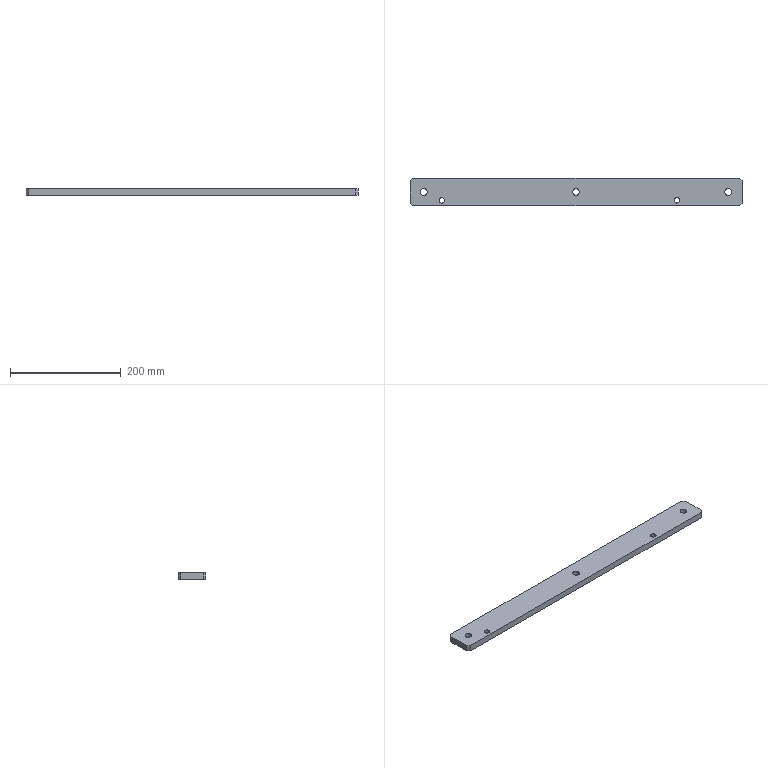Part | STEP file | [02]-6 | 1 solid | 20 faces | box 600 x 50 x 12 mm | volume 353444 mm3 | cylinder 10 | plane 10 | commonest cylinder face diameters 12 x6 10 x4
STEP:
#1=CARTESIAN_POINT('',(62.5,10.,12.));
#2=VERTEX_POINT('',#1);
#3=CARTESIAN_POINT('',(52.5,10.,12.));
#4=VERTEX_POINT('',#3);
#5=CARTESIAN_POINT('',(57.5,10.,12.));
#6=DIRECTION('',(0.,0.,-1.));
#7=DIRECTION('',(-1.,0.,0.));
#8=AXIS2_PLACEMENT_3D('',#5,#6,#7);
#9=CIRCLE('',#8,5.);
#10=EDGE_CURVE('',#2,#4,#9,.T.);
#11=ORIENTED_EDGE('',*,*,#10,.F.);
#12=CARTESIAN_POINT('',(62.5,10.,0.));
#13=VERTEX_POINT('',#12);
#14=CARTESIAN_POINT('',(62.5,10.,12.));
#15=DIRECTION('',(0.,0.,-1.));
#16=VECTOR('',#15,1000.);
#17=LINE('',#14,#16);
#18=EDGE_CURVE('',#2,#13,#17,.T.);
#19=ORIENTED_EDGE('',*,*,#18,.T.);
#20=CARTESIAN_POINT('',(52.5,10.,0.));
#21=VERTEX_POINT('',#20);
#22=CARTESIAN_POINT('',(57.5,10.,0.));
#23=DIRECTION('',(0.,0.,1.));
#24=DIRECTION('',(1.,0.,0.));
#25=AXIS2_PLACEMENT_3D('',#22,#23,#24);
#26=CIRCLE('',#25,5.);
#27=EDGE_CURVE('',#21,#13,#26,.T.);
#28=ORIENTED_EDGE('',*,*,#27,.F.);
#29=CARTESIAN_POINT('',(52.5,10.,12.));
#30=DIRECTION('',(0.,0.,-1.));
#31=VECTOR('',#30,1000.);
#32=LINE('',#29,#31);
#33=EDGE_CURVE('',#4,#21,#32,.T.);
#34=ORIENTED_EDGE('',*,*,#33,.F.);
#35=EDGE_LOOP('',(#11,#19,#28,#34));
#36=FACE_OUTER_BOUND('',#35,.T.);
#37=CARTESIAN_POINT('',(57.5,10.,12.));
#38=DIRECTION('',(0.,0.,-1.));
#39=DIRECTION('',(-1.,0.,0.));
#40=AXIS2_PLACEMENT_3D('',#37,#38,#39);
#41=CYLINDRICAL_SURFACE('',#40,5.);
#42=ADVANCED_FACE('',(#36),#41,.F.);
#43=CARTESIAN_POINT('',(482.5,15.,12.));
#44=VERTEX_POINT('',#43);
#45=CARTESIAN_POINT('',(482.5,5.,12.));
#46=VERTEX_POINT('',#45);
#47=CARTESIAN_POINT('',(482.5,10.,12.));
#48=DIRECTION('',(0.,0.,-1.));
#49=DIRECTION('',(0.,-1.,0.));
#50=AXIS2_PLACEMENT_3D('',#47,#48,#49);
#51=CIRCLE('',#50,5.);
#52=EDGE_CURVE('',#44,#46,#51,.T.);
#53=ORIENTED_EDGE('',*,*,#52,.F.);
#54=CARTESIAN_POINT('',(482.5,15.,0.));
#55=VERTEX_POINT('',#54);
#56=CARTESIAN_POINT('',(482.5,15.,12.));
#57=DIRECTION('',(0.,0.,-1.));
#58=VECTOR('',#57,1000.);
#59=LINE('',#56,#58);
#60=EDGE_CURVE('',#44,#55,#59,.T.);
#61=ORIENTED_EDGE('',*,*,#60,.T.);
#62=CARTESIAN_POINT('',(482.5,5.,0.));
#63=VERTEX_POINT('',#62);
#64=CARTESIAN_POINT('',(482.5,10.,0.));
#65=DIRECTION('',(0.,0.,1.));
#66=DIRECTION('',(0.,1.,0.));
#67=AXIS2_PLACEMENT_3D('',#64,#65,#66);
#68=CIRCLE('',#67,5.);
#69=EDGE_CURVE('',#63,#55,#68,.T.);
#70=ORIENTED_EDGE('',*,*,#69,.F.);
#71=CARTESIAN_POINT('',(482.5,5.,12.));
#72=DIRECTION('',(0.,0.,-1.));
#73=VECTOR('',#72,1000.);
#74=LINE('',#71,#73);
#75=EDGE_CURVE('',#46,#63,#74,.T.);
#76=ORIENTED_EDGE('',*,*,#75,.F.);
#77=EDGE_LOOP('',(#53,#61,#70,#76));
#78=FACE_OUTER_BOUND('',#77,.T.);
#79=CARTESIAN_POINT('',(482.5,10.,12.));
#80=DIRECTION('',(0.,0.,-1.));
#81=DIRECTION('',(0.,-1.,0.));
#82=AXIS2_PLACEMENT_3D('',#79,#80,#81);
#83=CYLINDRICAL_SURFACE('',#82,5.);
#84=ADVANCED_FACE('',(#78),#83,.F.);
#85=CARTESIAN_POINT('',(294.,25.,0.));
#86=VERTEX_POINT('',#85);
#87=CARTESIAN_POINT('',(306.,25.,0.));
#88=VERTEX_POINT('',#87);
#89=CARTESIAN_POINT('',(300.,25.,0.));
#90=DIRECTION('',(0.,0.,1.));
#91=DIRECTION('',(1.,0.,0.));
#92=AXIS2_PLACEMENT_3D('',#89,#90,#91);
#93=CIRCLE('',#92,6.);
#94=EDGE_CURVE('',#86,#88,#93,.T.);
#95=ORIENTED_EDGE('',*,*,#94,.F.);
#96=CARTESIAN_POINT('',(294.,25.,12.));
#97=VERTEX_POINT('',#96);
#98=CARTESIAN_POINT('',(294.,25.,0.));
#99=DIRECTION('',(0.,0.,1.));
#100=VECTOR('',#99,1000.);
#101=LINE('',#98,#100);
#102=EDGE_CURVE('',#86,#97,#101,.T.);
#103=ORIENTED_EDGE('',*,*,#102,.T.);
#104=CARTESIAN_POINT('',(306.,25.,12.));
#105=VERTEX_POINT('',#104);
#106=CARTESIAN_POINT('',(300.,25.,12.));
#107=DIRECTION('',(0.,0.,-1.));
#108=DIRECTION('',(-1.,0.,0.));
#109=AXIS2_PLACEMENT_3D('',#106,#107,#108);
#110=CIRCLE('',#109,6.);
#111=EDGE_CURVE('',#105,#97,#110,.T.);
#112=ORIENTED_EDGE('',*,*,#111,.F.);
#113=CARTESIAN_POINT('',(306.,25.,0.));
#114=DIRECTION('',(0.,0.,1.));
#115=VECTOR('',#114,1000.);
#116=LINE('',#113,#115);
#117=EDGE_CURVE('',#88,#105,#116,.T.);
#118=ORIENTED_EDGE('',*,*,#117,.F.);
#119=EDGE_LOOP('',(#95,#103,#112,#118));
#120=FACE_OUTER_BOUND('',#119,.T.);
#121=CARTESIAN_POINT('',(300.,25.,0.));
#122=DIRECTION('',(0.,0.,1.));
#123=DIRECTION('',(1.,0.,0.));
#124=AXIS2_PLACEMENT_3D('',#121,#122,#123);
#125=CYLINDRICAL_SURFACE('',#124,6.);
#126=ADVANCED_FACE('',(#120),#125,.F.);
#127=CARTESIAN_POINT('',(19.,25.,0.));
#128=VERTEX_POINT('',#127);
#129=CARTESIAN_POINT('',(31.,25.,0.));
#130=VERTEX_POINT('',#129);
#131=CARTESIAN_POINT('',(25.,25.,0.));
#132=DIRECTION('',(0.,0.,1.));
#133=DIRECTION('',(1.,0.,0.));
#134=AXIS2_PLACEMENT_3D('',#131,#132,#133);
#135=CIRCLE('',#134,6.);
#136=EDGE_CURVE('',#128,#130,#135,.T.);
#137=ORIENTED_EDGE('',*,*,#136,.F.);
#138=CARTESIAN_POINT('',(19.,25.,12.));
#139=VERTEX_POINT('',#138);
#140=CARTESIAN_POINT('',(19.,25.,0.));
#141=DIRECTION('',(0.,0.,1.));
#142=VECTOR('',#141,1000.);
#143=LINE('',#140,#142);
#144=EDGE_CURVE('',#128,#139,#143,.T.);
#145=ORIENTED_EDGE('',*,*,#144,.T.);
#146=CARTESIAN_POINT('',(31.,25.,12.));
#147=VERTEX_POINT('',#146);
#148=CARTESIAN_POINT('',(25.,25.,12.));
#149=DIRECTION('',(0.,0.,-1.));
#150=DIRECTION('',(-1.,0.,0.));
#151=AXIS2_PLACEMENT_3D('',#148,#149,#150);
#152=CIRCLE('',#151,6.);
#153=EDGE_CURVE('',#147,#139,#152,.T.);
#154=ORIENTED_EDGE('',*,*,#153,.F.);
#155=CARTESIAN_POINT('',(31.,25.,0.));
#156=DIRECTION('',(0.,0.,1.));
#157=VECTOR('',#156,1000.);
#158=LINE('',#155,#157);
#159=EDGE_CURVE('',#130,#147,#158,.T.);
#160=ORIENTED_EDGE('',*,*,#159,.F.);
#161=EDGE_LOOP('',(#137,#145,#154,#160));
#162=FACE_OUTER_BOUND('',#161,.T.);
#163=CARTESIAN_POINT('',(25.,25.,0.));
#164=DIRECTION('',(0.,0.,1.));
#165=DIRECTION('',(1.,0.,0.));
#166=AXIS2_PLACEMENT_3D('',#163,#164,#165);
#167=CYLINDRICAL_SURFACE('',#166,6.);
#168=ADVANCED_FACE('',(#162),#167,.F.);
#169=CARTESIAN_POINT('',(569.,25.,0.));
#170=VERTEX_POINT('',#169);
#171=CARTESIAN_POINT('',(581.,25.,0.));
#172=VERTEX_POINT('',#171);
#173=CARTESIAN_POINT('',(575.,25.,0.));
#174=DIRECTION('',(0.,0.,1.));
#175=DIRECTION('',(1.,0.,0.));
#176=AXIS2_PLACEMENT_3D('',#173,#174,#175);
#177=CIRCLE('',#176,6.);
#178=EDGE_CURVE('',#170,#172,#177,.T.);
#179=ORIENTED_EDGE('',*,*,#178,.F.);
#180=CARTESIAN_POINT('',(569.,25.,12.));
#181=VERTEX_POINT('',#180);
#182=CARTESIAN_POINT('',(569.,25.,0.));
#183=DIRECTION('',(0.,0.,1.));
#184=VECTOR('',#183,1000.);
#185=LINE('',#182,#184);
#186=EDGE_CURVE('',#170,#181,#185,.T.);
#187=ORIENTED_EDGE('',*,*,#186,.T.);
#188=CARTESIAN_POINT('',(581.,25.,12.));
#189=VERTEX_POINT('',#188);
#190=CARTESIAN_POINT('',(575.,25.,12.));
#191=DIRECTION('',(0.,0.,-1.));
#192=DIRECTION('',(-1.,0.,0.));
#193=AXIS2_PLACEMENT_3D('',#190,#191,#192);
#194=CIRCLE('',#193,6.);
#195=EDGE_CURVE('',#189,#181,#194,.T.);
#196=ORIENTED_EDGE('',*,*,#195,.F.);
#197=CARTESIAN_POINT('',(581.,25.,0.));
#198=DIRECTION('',(0.,0.,1.));
#199=VECTOR('',#198,1000.);
#200=LINE('',#197,#199);
#201=EDGE_CURVE('',#172,#189,#200,.T.);
#202=ORIENTED_EDGE('',*,*,#201,.F.);
#203=EDGE_LOOP('',(#179,#187,#196,#202));
#204=FACE_OUTER_BOUND('',#203,.T.);
#205=CARTESIAN_POINT('',(575.,25.,0.));
#206=DIRECTION('',(0.,0.,1.));
#207=DIRECTION('',(1.,0.,0.));
#208=AXIS2_PLACEMENT_3D('',#205,#206,#207);
#209=CYLINDRICAL_SURFACE('',#208,6.);
#210=ADVANCED_FACE('',(#204),#209,.F.);
#211=ORIENTED_EDGE('',*,*,#27,.T.);
#212=CARTESIAN_POINT('',(57.5,10.,0.));
#213=DIRECTION('',(0.,0.,1.));
#214=DIRECTION('',(1.,0.,0.));
#215=AXIS2_PLACEMENT_3D('',#212,#213,#214);
#216=CIRCLE('',#215,5.);
#217=EDGE_CURVE('',#13,#21,#216,.T.);
#218=ORIENTED_EDGE('',*,*,#217,.T.);
#219=EDGE_LOOP('',(#211,#218));
#220=FACE_BOUND('',#219,.T.);
#221=ORIENTED_EDGE('',*,*,#69,.T.);
#222=CARTESIAN_POINT('',(482.5,10.,0.));
#223=DIRECTION('',(0.,0.,1.));
#224=DIRECTION('',(0.,1.,0.));
#225=AXIS2_PLACEMENT_3D('',#222,#223,#224);
#226=CIRCLE('',#225,5.);
#227=EDGE_CURVE('',#55,#63,#226,.T.);
#228=ORIENTED_EDGE('',*,*,#227,.T.);
#229=EDGE_LOOP('',(#221,#228));
#230=FACE_BOUND('',#229,.T.);
#231=CARTESIAN_POINT('',(300.,25.,0.));
#232=DIRECTION('',(0.,0.,1.));
#233=DIRECTION('',(1.,0.,0.));
#234=AXIS2_PLACEMENT_3D('',#231,#232,#233);
#235=CIRCLE('',#234,6.);
#236=EDGE_CURVE('',#88,#86,#235,.T.);
#237=ORIENTED_EDGE('',*,*,#236,.T.);
#238=ORIENTED_EDGE('',*,*,#94,.T.);
#239=EDGE_LOOP('',(#237,#238));
#240=FACE_BOUND('',#239,.T.);
#241=CARTESIAN_POINT('',(25.,25.,0.));
#242=DIRECTION('',(0.,0.,1.));
#243=DIRECTION('',(1.,0.,0.));
#244=AXIS2_PLACEMENT_3D('',#241,#242,#243);
#245=CIRCLE('',#244,6.);
#246=EDGE_CURVE('',#130,#128,#245,.T.);
#247=ORIENTED_EDGE('',*,*,#246,.T.);
#248=ORIENTED_EDGE('',*,*,#136,.T.);
#249=EDGE_LOOP('',(#247,#248));
#250=FACE_BOUND('',#249,.T.);
#251=CARTESIAN_POINT('',(575.,25.,0.));
#252=DIRECTION('',(0.,0.,1.));
#253=DIRECTION('',(1.,0.,0.));
#254=AXIS2_PLACEMENT_3D('',#251,#252,#253);
#255=CIRCLE('',#254,6.);
#256=EDGE_CURVE('',#172,#170,#255,.T.);
#257=ORIENTED_EDGE('',*,*,#256,.T.);
#258=ORIENTED_EDGE('',*,*,#178,.T.);
#259=EDGE_LOOP('',(#257,#258));
#260=FACE_BOUND('',#259,.T.);
#261=CARTESIAN_POINT('',(0.,45.,0.));
#262=VERTEX_POINT('',#261);
#263=CARTESIAN_POINT('',(0.,5.,0.));
#264=VERTEX_POINT('',#263);
#265=CARTESIAN_POINT('',(0.,25.,0.));
#266=DIRECTION('',(0.,-1.,0.));
#267=VECTOR('',#266,1000.);
#268=LINE('',#265,#267);
#269=EDGE_CURVE('',#262,#264,#268,.T.);
#270=ORIENTED_EDGE('',*,*,#269,.F.);
#271=CARTESIAN_POINT('',(5.,50.,0.));
#272=VERTEX_POINT('',#271);
#273=CARTESIAN_POINT('',(140.,185.,0.));
#274=DIRECTION('',(0.7071,0.7071,0.));
#275=VECTOR('',#274,1000.);
#276=LINE('',#273,#275);
#277=EDGE_CURVE('',#262,#272,#276,.T.);
#278=ORIENTED_EDGE('',*,*,#277,.T.);
#279=CARTESIAN_POINT('',(595.,50.,0.));
#280=VERTEX_POINT('',#279);
#281=CARTESIAN_POINT('',(300.,50.,0.));
#282=DIRECTION('',(-1.,0.,0.));
#283=VECTOR('',#282,1000.);
#284=LINE('',#281,#283);
#285=EDGE_CURVE('',#280,#272,#284,.T.);
#286=ORIENTED_EDGE('',*,*,#285,.F.);
#287=CARTESIAN_POINT('',(600.,45.,0.));
#288=VERTEX_POINT('',#287);
#289=CARTESIAN_POINT('',(460.,185.,0.));
#290=DIRECTION('',(0.7071,-0.7071,0.));
#291=VECTOR('',#290,1000.);
#292=LINE('',#289,#291);
#293=EDGE_CURVE('',#280,#288,#292,.T.);
#294=ORIENTED_EDGE('',*,*,#293,.T.);
#295=CARTESIAN_POINT('',(600.,5.,0.));
#296=VERTEX_POINT('',#295);
#297=CARTESIAN_POINT('',(600.,25.,0.));
#298=DIRECTION('',(0.,1.,0.));
#299=VECTOR('',#298,1000.);
#300=LINE('',#297,#299);
#301=EDGE_CURVE('',#296,#288,#300,.T.);
#302=ORIENTED_EDGE('',*,*,#301,.F.);
#303=CARTESIAN_POINT('',(595.,0.,0.));
#304=VERTEX_POINT('',#303);
#305=CARTESIAN_POINT('',(460.,-135.,0.));
#306=DIRECTION('',(-0.7071,-0.7071,0.));
#307=VECTOR('',#306,1000.);
#308=LINE('',#305,#307);
#309=EDGE_CURVE('',#296,#304,#308,.T.);
#310=ORIENTED_EDGE('',*,*,#309,.T.);
#311=CARTESIAN_POINT('',(5.,0.,0.));
#312=VERTEX_POINT('',#311);
#313=CARTESIAN_POINT('',(300.,0.,0.));
#314=DIRECTION('',(1.,0.,0.));
#315=VECTOR('',#314,1000.);
#316=LINE('',#313,#315);
#317=EDGE_CURVE('',#312,#304,#316,.T.);
#318=ORIENTED_EDGE('',*,*,#317,.F.);
#319=CARTESIAN_POINT('',(140.,-135.,0.));
#320=DIRECTION('',(-0.7071,0.7071,0.));
#321=VECTOR('',#320,1000.);
#322=LINE('',#319,#321);
#323=EDGE_CURVE('',#312,#264,#322,.T.);
#324=ORIENTED_EDGE('',*,*,#323,.T.);
#325=EDGE_LOOP('',(#270,#278,#286,#294,#302,#310,#318,#324));
#326=FACE_OUTER_BOUND('',#325,.T.);
#327=CARTESIAN_POINT('',(300.,25.,0.));
#328=DIRECTION('',(0.,0.,-1.));
#329=DIRECTION('',(-1.,0.,0.));
#330=AXIS2_PLACEMENT_3D('',#327,#328,#329);
#331=PLANE('',#330);
#332=ADVANCED_FACE('',(#220,#230,#240,#250,#260,#326),#331,.T.);
#333=CARTESIAN_POINT('',(595.,0.,12.));
#334=VERTEX_POINT('',#333);
#335=CARTESIAN_POINT('',(5.,0.,12.));
#336=VERTEX_POINT('',#335);
#337=CARTESIAN_POINT('',(300.,0.,12.));
#338=DIRECTION('',(-1.,0.,0.));
#339=VECTOR('',#338,1000.);
#340=LINE('',#337,#339);
#341=EDGE_CURVE('',#334,#336,#340,.T.);
#342=ORIENTED_EDGE('',*,*,#341,.T.);
#343=CARTESIAN_POINT('',(5.,0.,12.));
#344=DIRECTION('',(0.,0.,-1.));
#345=VECTOR('',#344,1000.);
#346=LINE('',#343,#345);
#347=EDGE_CURVE('',#336,#312,#346,.T.);
#348=ORIENTED_EDGE('',*,*,#347,.T.);
#349=ORIENTED_EDGE('',*,*,#317,.T.);
#350=CARTESIAN_POINT('',(595.,0.,12.));
#351=DIRECTION('',(0.,0.,1.));
#352=VECTOR('',#351,1000.);
#353=LINE('',#350,#352);
#354=EDGE_CURVE('',#304,#334,#353,.T.);
#355=ORIENTED_EDGE('',*,*,#354,.T.);
#356=EDGE_LOOP('',(#342,#348,#349,#355));
#357=FACE_OUTER_BOUND('',#356,.T.);
#358=CARTESIAN_POINT('',(300.,0.,12.));
#359=DIRECTION('',(0.,-1.,0.));
#360=DIRECTION('',(0.,0.,1.));
#361=AXIS2_PLACEMENT_3D('',#358,#359,#360);
#362=PLANE('',#361);
#363=ADVANCED_FACE('',(#357),#362,.T.);
#364=ORIENTED_EDGE('',*,*,#301,.T.);
#365=CARTESIAN_POINT('',(600.,45.,12.));
#366=VERTEX_POINT('',#365);
#367=CARTESIAN_POINT('',(600.,45.,12.));
#368=DIRECTION('',(0.,0.,1.));
#369=VECTOR('',#368,1000.);
#370=LINE('',#367,#369);
#371=EDGE_CURVE('',#288,#366,#370,.T.);
#372=ORIENTED_EDGE('',*,*,#371,.T.);
#373=CARTESIAN_POINT('',(600.,5.,12.));
#374=VERTEX_POINT('',#373);
#375=CARTESIAN_POINT('',(600.,25.,12.));
#376=DIRECTION('',(0.,-1.,0.));
#377=VECTOR('',#376,1000.);
#378=LINE('',#375,#377);
#379=EDGE_CURVE('',#366,#374,#378,.T.);
#380=ORIENTED_EDGE('',*,*,#379,.T.);
#381=CARTESIAN_POINT('',(600.,5.,12.));
#382=DIRECTION('',(0.,0.,-1.));
#383=VECTOR('',#382,1000.);
#384=LINE('',#381,#383);
#385=EDGE_CURVE('',#374,#296,#384,.T.);
#386=ORIENTED_EDGE('',*,*,#385,.T.);
#387=EDGE_LOOP('',(#364,#372,#380,#386));
#388=FACE_OUTER_BOUND('',#387,.T.);
#389=CARTESIAN_POINT('',(600.,25.,12.));
#390=DIRECTION('',(1.,0.,0.));
#391=DIRECTION('',(0.,0.,-1.));
#392=AXIS2_PLACEMENT_3D('',#389,#390,#391);
#393=PLANE('',#392);
#394=ADVANCED_FACE('',(#388),#393,.T.);
#395=ORIENTED_EDGE('',*,*,#285,.T.);
#396=CARTESIAN_POINT('',(5.,50.,12.));
#397=VERTEX_POINT('',#396);
#398=CARTESIAN_POINT('',(5.,50.,12.));
#399=DIRECTION('',(0.,0.,1.));
#400=VECTOR('',#399,1000.);
#401=LINE('',#398,#400);
#402=EDGE_CURVE('',#272,#397,#401,.T.);
#403=ORIENTED_EDGE('',*,*,#402,.T.);
#404=CARTESIAN_POINT('',(595.,50.,12.));
#405=VERTEX_POINT('',#404);
#406=CARTESIAN_POINT('',(300.,50.,12.));
#407=DIRECTION('',(1.,0.,0.));
#408=VECTOR('',#407,1000.);
#409=LINE('',#406,#408);
#410=EDGE_CURVE('',#397,#405,#409,.T.);
#411=ORIENTED_EDGE('',*,*,#410,.T.);
#412=CARTESIAN_POINT('',(595.,50.,12.));
#413=DIRECTION('',(0.,0.,-1.));
#414=VECTOR('',#413,1000.);
#415=LINE('',#412,#414);
#416=EDGE_CURVE('',#405,#280,#415,.T.);
#417=ORIENTED_EDGE('',*,*,#416,.T.);
#418=EDGE_LOOP('',(#395,#403,#411,#417));
#419=FACE_OUTER_BOUND('',#418,.T.);
#420=CARTESIAN_POINT('',(300.,50.,12.));
#421=DIRECTION('',(0.,1.,0.));
#422=DIRECTION('',(0.,0.,-1.));
#423=AXIS2_PLACEMENT_3D('',#420,#421,#422);
#424=PLANE('',#423);
#425=ADVANCED_FACE('',(#419),#424,.T.);
#426=CARTESIAN_POINT('',(57.5,10.,12.));
#427=DIRECTION('',(0.,0.,-1.));
#428=DIRECTION('',(-1.,0.,0.));
#429=AXIS2_PLACEMENT_3D('',#426,#427,#428);
#430=CIRCLE('',#429,5.);
#431=EDGE_CURVE('',#4,#2,#430,.T.);
#432=ORIENTED_EDGE('',*,*,#431,.T.);
#433=ORIENTED_EDGE('',*,*,#10,.T.);
#434=EDGE_LOOP('',(#432,#433));
#435=FACE_BOUND('',#434,.T.);
#436=CARTESIAN_POINT('',(482.5,10.,12.));
#437=DIRECTION('',(0.,0.,-1.));
#438=DIRECTION('',(0.,-1.,0.));
#439=AXIS2_PLACEMENT_3D('',#436,#437,#438);
#440=CIRCLE('',#439,5.);
#441=EDGE_CURVE('',#46,#44,#440,.T.);
#442=ORIENTED_EDGE('',*,*,#441,.T.);
#443=ORIENTED_EDGE('',*,*,#52,.T.);
#444=EDGE_LOOP('',(#442,#443));
#445=FACE_BOUND('',#444,.T.);
#446=ORIENTED_EDGE('',*,*,#111,.T.);
#447=CARTESIAN_POINT('',(300.,25.,12.));
#448=DIRECTION('',(0.,0.,-1.));
#449=DIRECTION('',(-1.,0.,0.));
#450=AXIS2_PLACEMENT_3D('',#447,#448,#449);
#451=CIRCLE('',#450,6.);
#452=EDGE_CURVE('',#97,#105,#451,.T.);
#453=ORIENTED_EDGE('',*,*,#452,.T.);
#454=EDGE_LOOP('',(#446,#453));
#455=FACE_BOUND('',#454,.T.);
#456=ORIENTED_EDGE('',*,*,#153,.T.);
#457=CARTESIAN_POINT('',(25.,25.,12.));
#458=DIRECTION('',(0.,0.,-1.));
#459=DIRECTION('',(-1.,0.,0.));
#460=AXIS2_PLACEMENT_3D('',#457,#458,#459);
#461=CIRCLE('',#460,6.);
#462=EDGE_CURVE('',#139,#147,#461,.T.);
#463=ORIENTED_EDGE('',*,*,#462,.T.);
#464=EDGE_LOOP('',(#456,#463));
#465=FACE_BOUND('',#464,.T.);
#466=ORIENTED_EDGE('',*,*,#195,.T.);
#467=CARTESIAN_POINT('',(575.,25.,12.));
#468=DIRECTION('',(0.,0.,-1.));
#469=DIRECTION('',(-1.,0.,0.));
#470=AXIS2_PLACEMENT_3D('',#467,#468,#469);
#471=CIRCLE('',#470,6.);
#472=EDGE_CURVE('',#181,#189,#471,.T.);
#473=ORIENTED_EDGE('',*,*,#472,.T.);
#474=EDGE_LOOP('',(#466,#473));
#475=FACE_BOUND('',#474,.T.);
#476=ORIENTED_EDGE('',*,*,#410,.F.);
#477=CARTESIAN_POINT('',(0.,45.,12.));
#478=VERTEX_POINT('',#477);
#479=CARTESIAN_POINT('',(140.,185.,12.));
#480=DIRECTION('',(-0.7071,-0.7071,0.));
#481=VECTOR('',#480,1000.);
#482=LINE('',#479,#481);
#483=EDGE_CURVE('',#397,#478,#482,.T.);
#484=ORIENTED_EDGE('',*,*,#483,.T.);
#485=CARTESIAN_POINT('',(0.,5.,12.));
#486=VERTEX_POINT('',#485);
#487=CARTESIAN_POINT('',(0.,25.,12.));
#488=DIRECTION('',(0.,1.,0.));
#489=VECTOR('',#488,1000.);
#490=LINE('',#487,#489);
#491=EDGE_CURVE('',#486,#478,#490,.T.);
#492=ORIENTED_EDGE('',*,*,#491,.F.);
#493=CARTESIAN_POINT('',(140.,-135.,12.));
#494=DIRECTION('',(0.7071,-0.7071,0.));
#495=VECTOR('',#494,1000.);
#496=LINE('',#493,#495);
#497=EDGE_CURVE('',#486,#336,#496,.T.);
#498=ORIENTED_EDGE('',*,*,#497,.T.);
#499=ORIENTED_EDGE('',*,*,#341,.F.);
#500=CARTESIAN_POINT('',(460.,-135.,12.));
#501=DIRECTION('',(0.7071,0.7071,0.));
#502=VECTOR('',#501,1000.);
#503=LINE('',#500,#502);
#504=EDGE_CURVE('',#334,#374,#503,.T.);
#505=ORIENTED_EDGE('',*,*,#504,.T.);
#506=ORIENTED_EDGE('',*,*,#379,.F.);
#507=CARTESIAN_POINT('',(460.,185.,12.));
#508=DIRECTION('',(-0.7071,0.7071,0.));
#509=VECTOR('',#508,1000.);
#510=LINE('',#507,#509);
#511=EDGE_CURVE('',#366,#405,#510,.T.);
#512=ORIENTED_EDGE('',*,*,#511,.T.);
#513=EDGE_LOOP('',(#476,#484,#492,#498,#499,#505,#506,#512));
#514=FACE_OUTER_BOUND('',#513,.T.);
#515=CARTESIAN_POINT('',(300.,25.,12.));
#516=DIRECTION('',(0.,0.,1.));
#517=DIRECTION('',(1.,0.,0.));
#518=AXIS2_PLACEMENT_3D('',#515,#516,#517);
#519=PLANE('',#518);
#520=ADVANCED_FACE('',(#435,#445,#455,#465,#475,#514),#519,.T.);
#521=ORIENTED_EDGE('',*,*,#491,.T.);
#522=CARTESIAN_POINT('',(0.,45.,12.));
#523=DIRECTION('',(0.,0.,-1.));
#524=VECTOR('',#523,1000.);
#525=LINE('',#522,#524);
#526=EDGE_CURVE('',#478,#262,#525,.T.);
#527=ORIENTED_EDGE('',*,*,#526,.T.);
#528=ORIENTED_EDGE('',*,*,#269,.T.);
#529=CARTESIAN_POINT('',(0.,5.,12.));
#530=DIRECTION('',(0.,0.,1.));
#531=VECTOR('',#530,1000.);
#532=LINE('',#529,#531);
#533=EDGE_CURVE('',#264,#486,#532,.T.);
#534=ORIENTED_EDGE('',*,*,#533,.T.);
#535=EDGE_LOOP('',(#521,#527,#528,#534));
#536=FACE_OUTER_BOUND('',#535,.T.);
#537=CARTESIAN_POINT('',(0.,25.,12.));
#538=DIRECTION('',(-1.,0.,0.));
#539=DIRECTION('',(0.,0.,1.));
#540=AXIS2_PLACEMENT_3D('',#537,#538,#539);
#541=PLANE('',#540);
#542=ADVANCED_FACE('',(#536),#541,.T.);
#543=ORIENTED_EDGE('',*,*,#186,.F.);
#544=ORIENTED_EDGE('',*,*,#256,.F.);
#545=ORIENTED_EDGE('',*,*,#201,.T.);
#546=ORIENTED_EDGE('',*,*,#472,.F.);
#547=EDGE_LOOP('',(#543,#544,#545,#546));
#548=FACE_OUTER_BOUND('',#547,.T.);
#549=CARTESIAN_POINT('',(575.,25.,0.));
#550=DIRECTION('',(0.,0.,1.));
#551=DIRECTION('',(1.,0.,0.));
#552=AXIS2_PLACEMENT_3D('',#549,#550,#551);
#553=CYLINDRICAL_SURFACE('',#552,6.);
#554=ADVANCED_FACE('',(#548),#553,.F.);
#555=ORIENTED_EDGE('',*,*,#144,.F.);
#556=ORIENTED_EDGE('',*,*,#246,.F.);
#557=ORIENTED_EDGE('',*,*,#159,.T.);
#558=ORIENTED_EDGE('',*,*,#462,.F.);
#559=EDGE_LOOP('',(#555,#556,#557,#558));
#560=FACE_OUTER_BOUND('',#559,.T.);
#561=CARTESIAN_POINT('',(25.,25.,0.));
#562=DIRECTION('',(0.,0.,1.));
#563=DIRECTION('',(1.,0.,0.));
#564=AXIS2_PLACEMENT_3D('',#561,#562,#563);
#565=CYLINDRICAL_SURFACE('',#564,6.);
#566=ADVANCED_FACE('',(#560),#565,.F.);
#567=ORIENTED_EDGE('',*,*,#102,.F.);
#568=ORIENTED_EDGE('',*,*,#236,.F.);
#569=ORIENTED_EDGE('',*,*,#117,.T.);
#570=ORIENTED_EDGE('',*,*,#452,.F.);
#571=EDGE_LOOP('',(#567,#568,#569,#570));
#572=FACE_OUTER_BOUND('',#571,.T.);
#573=CARTESIAN_POINT('',(300.,25.,0.));
#574=DIRECTION('',(0.,0.,1.));
#575=DIRECTION('',(1.,0.,0.));
#576=AXIS2_PLACEMENT_3D('',#573,#574,#575);
#577=CYLINDRICAL_SURFACE('',#576,6.);
#578=ADVANCED_FACE('',(#572),#577,.F.);
#579=ORIENTED_EDGE('',*,*,#504,.F.);
#580=ORIENTED_EDGE('',*,*,#354,.F.);
#581=ORIENTED_EDGE('',*,*,#309,.F.);
#582=ORIENTED_EDGE('',*,*,#385,.F.);
#583=EDGE_LOOP('',(#579,#580,#581,#582));
#584=FACE_OUTER_BOUND('',#583,.T.);
#585=CARTESIAN_POINT('',(600.,5.,12.));
#586=DIRECTION('',(-0.7071,0.7071,0.));
#587=DIRECTION('',(0.,0.,-1.));
#588=AXIS2_PLACEMENT_3D('',#585,#586,#587);
#589=PLANE('',#588);
#590=ADVANCED_FACE('',(#584),#589,.F.);
#591=ORIENTED_EDGE('',*,*,#511,.F.);
#592=ORIENTED_EDGE('',*,*,#371,.F.);
#593=ORIENTED_EDGE('',*,*,#293,.F.);
#594=ORIENTED_EDGE('',*,*,#416,.F.);
#595=EDGE_LOOP('',(#591,#592,#593,#594));
#596=FACE_OUTER_BOUND('',#595,.T.);
#597=CARTESIAN_POINT('',(595.,50.,12.));
#598=DIRECTION('',(-0.7071,-0.7071,0.));
#599=DIRECTION('',(0.,0.,-1.));
#600=AXIS2_PLACEMENT_3D('',#597,#598,#599);
#601=PLANE('',#600);
#602=ADVANCED_FACE('',(#596),#601,.F.);
#603=ORIENTED_EDGE('',*,*,#497,.F.);
#604=ORIENTED_EDGE('',*,*,#533,.F.);
#605=ORIENTED_EDGE('',*,*,#323,.F.);
#606=ORIENTED_EDGE('',*,*,#347,.F.);
#607=EDGE_LOOP('',(#603,#604,#605,#606));
#608=FACE_OUTER_BOUND('',#607,.T.);
#609=CARTESIAN_POINT('',(5.,0.,12.));
#610=DIRECTION('',(0.7071,0.7071,0.));
#611=DIRECTION('',(0.,0.,-1.));
#612=AXIS2_PLACEMENT_3D('',#609,#610,#611);
#613=PLANE('',#612);
#614=ADVANCED_FACE('',(#608),#613,.F.);
#615=ORIENTED_EDGE('',*,*,#483,.F.);
#616=ORIENTED_EDGE('',*,*,#402,.F.);
#617=ORIENTED_EDGE('',*,*,#277,.F.);
#618=ORIENTED_EDGE('',*,*,#526,.F.);
#619=EDGE_LOOP('',(#615,#616,#617,#618));
#620=FACE_OUTER_BOUND('',#619,.T.);
#621=CARTESIAN_POINT('',(0.,45.,12.));
#622=DIRECTION('',(0.7071,-0.7071,0.));
#623=DIRECTION('',(0.,0.,-1.));
#624=AXIS2_PLACEMENT_3D('',#621,#622,#623);
#625=PLANE('',#624);
#626=ADVANCED_FACE('',(#620),#625,.F.);
#627=ORIENTED_EDGE('',*,*,#60,.F.);
#628=ORIENTED_EDGE('',*,*,#441,.F.);
#629=ORIENTED_EDGE('',*,*,#75,.T.);
#630=ORIENTED_EDGE('',*,*,#227,.F.);
#631=EDGE_LOOP('',(#627,#628,#629,#630));
#632=FACE_OUTER_BOUND('',#631,.T.);
#633=CARTESIAN_POINT('',(482.5,10.,12.));
#634=DIRECTION('',(0.,0.,-1.));
#635=DIRECTION('',(0.,-1.,0.));
#636=AXIS2_PLACEMENT_3D('',#633,#634,#635);
#637=CYLINDRICAL_SURFACE('',#636,5.);
#638=ADVANCED_FACE('',(#632),#637,.F.);
#639=ORIENTED_EDGE('',*,*,#18,.F.);
#640=ORIENTED_EDGE('',*,*,#431,.F.);
#641=ORIENTED_EDGE('',*,*,#33,.T.);
#642=ORIENTED_EDGE('',*,*,#217,.F.);
#643=EDGE_LOOP('',(#639,#640,#641,#642));
#644=FACE_OUTER_BOUND('',#643,.T.);
#645=CARTESIAN_POINT('',(57.5,10.,12.));
#646=DIRECTION('',(0.,0.,-1.));
#647=DIRECTION('',(-1.,0.,0.));
#648=AXIS2_PLACEMENT_3D('',#645,#646,#647);
#649=CYLINDRICAL_SURFACE('',#648,5.);
#650=ADVANCED_FACE('',(#644),#649,.F.);
#651=CLOSED_SHELL('',(#42,#84,#126,#168,#210,#332,#363,#394,#425,#520,#542,#554,#566,#578,#590,#602,#614,#626,#638,#650));
#652=MANIFOLD_SOLID_BREP('',#651);
#653=CARTESIAN_POINT('',(0.,0.,0.));
#654=DIRECTION('',(0.,0.,1.));
#655=DIRECTION('',(1.,0.,0.));
#656=AXIS2_PLACEMENT_3D('',#653,#654,#655);
#657=(LENGTH_UNIT()NAMED_UNIT(*)SI_UNIT(.MILLI.,.METRE.));
#658=UNCERTAINTY_MEASURE_WITH_UNIT(LENGTH_MEASURE(0.00001),#657,'','');
#659=(NAMED_UNIT(*)PLANE_ANGLE_UNIT()SI_UNIT($,.RADIAN.));
#660=(NAMED_UNIT(*)SI_UNIT($,.STERADIAN.)SOLID_ANGLE_UNIT());
#661=(GEOMETRIC_REPRESENTATION_CONTEXT(3)GLOBAL_UNCERTAINTY_ASSIGNED_CONTEXT((#658))GLOBAL_UNIT_ASSIGNED_CONTEXT((#657,#659,#660))REPRESENTATION_CONTEXT('',''));
#662=ADVANCED_BREP_SHAPE_REPRESENTATION('',(#652,#656),#661);